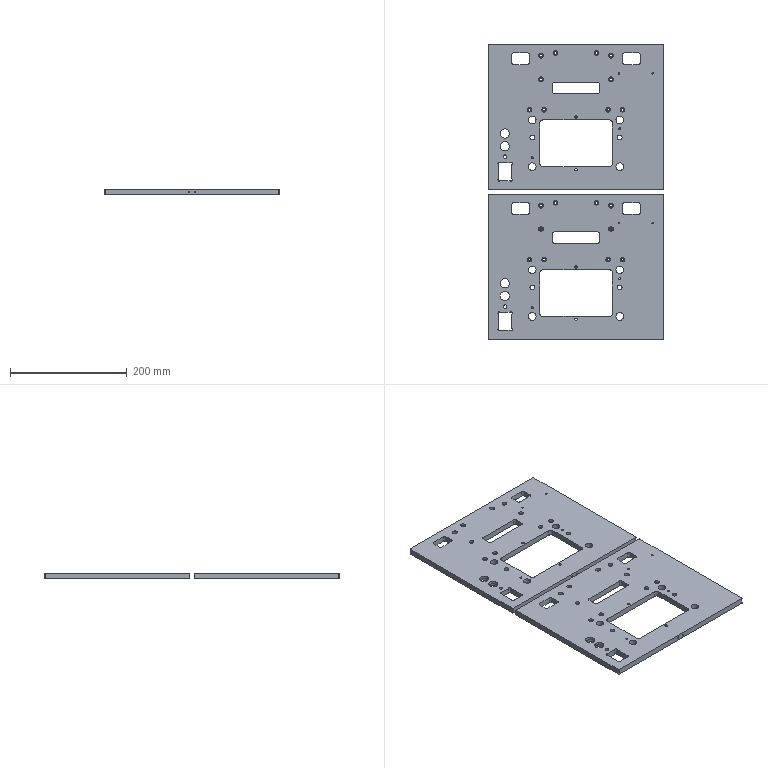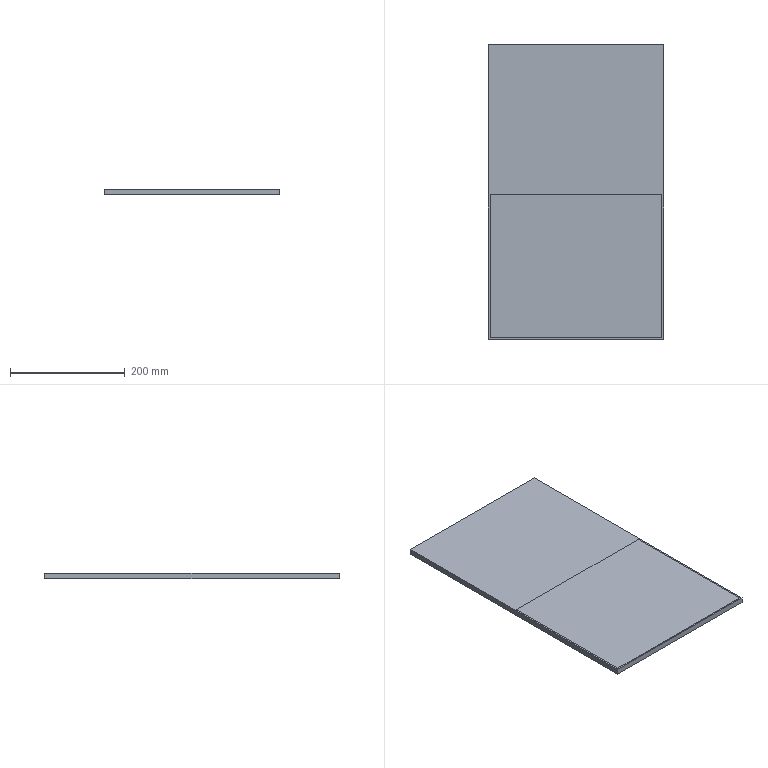CAM job | NX | 3-axis milling, drilling | part box 300 x 507 x 10 mm | stock box 306 x 513 x 10 mm
Tools:
number,name,description,diameter,corner_radius,flute_length,length,flutes
2,D4A45,Milling Tool-5 Parameters,4.0,0.0,2.0,2.0,2
6,D6,Milling Tool-5 Parameters,6.0,0.0,50.0,75.0,2
4,D4,Milling Tool-5 Parameters,4.0,0.0,50.0,75.0,2
13,3.3ZT,Drilling Tool,3.3,0.0,35.0,50.0,2
11,2.5ZT,Drilling Tool,2.5,0.0,35.0,50.0,2
16,4.5ZT,Drilling Tool,4.5,0.0,35.0,50.0,2
14,4.2ZT,Drilling Tool,4.2,0.0,35.0,50.0,2
3,D3,Milling Tool-5 Parameters,3.0,0.0,50.0,75.0,2
Operations:
program,operation,operation_type,tool,method,geometry_group,spindle_rpm,surface_speed,feed_per_tooth,feed_cut,feed_plunge,cut_length_mm,path_length_mm,cut_time_min,machine_time_min
VACUUM1,ZLEVEL_PROFILE_1_COPY_1_COPY_COPY,ZLevelMilling,D4A45,METHOD,A,9500.0,179.0,0.0526,1000.0,100.0,5201.024,17082.464,5.201,6.389
VACUUM1,ZLEVEL_PROFILE_COPY_COPY_1_COPY,ZLevelMilling,D6,METHOD,A,9500.0,179.0,0.1158,2200.0,1000.0,44810.694,45457.393,20.41,20.474
VACUUM1,HOLE_MILLING_COPY,CylinderMilling,D6,METHOD,A,9500.0,179.0,0.0789,1500.0,100.0,1620.814,3835.318,1.081,1.302
VACUUM1,ZLEVEL_PROFILE_COPY_COPY_1_COPY_COPY,ZLevelMilling,D6,METHOD,A,9500.0,179.0,0.0868,1650.0,1000.0,28912.267,30385.631,17.642,17.79
VACUUM1,ZLEVEL_PROFILE_COPY_COPY_COPY_COPY_COPY,ZLevelMilling,D4,MILL_FINISH,A,9500.0,119.0,0.0632,1200.0,1000.0,2228.073,2973.01,1.857,1.932
2,DRILLING_COPY,Operation,D4A45,METHOD,B,5000.0,62.0,0.025,250.0,0.0,140.0,1498.085,0.56,0.6958
2,DRILLING_COPY_COPY_COPY_COPY_COPY,Operation,3.3ZT,METHOD,B,1910.0,21.0,0.0471,180.0,0.0,30.983,283.108,0.1721,0.1973
2,DRILLING_COPY_COPY_COPY_COPY_COPY_COPY_1,Operation,3.3ZT,METHOD,B,1910.0,21.0,0.0471,180.0,0.0,30.983,215.016,0.1721,0.1905
2,DRILLING_COPY_COPY_COPY_COPY_COPY_COPY,Operation,2.5ZT,METHOD,B,1910.0,21.0,0.0471,180.0,0.0,30.502,182.082,0.1695,0.1846
2,DRILLING_COPY_COPY_COPY_COPY_COPY_COPY_COPY_1,Operation,2.5ZT,METHOD,B,1910.0,21.0,0.0471,180.0,0.0,28.506,404.23,0.1584,0.1959
2,DRILLING_COPY_COPY_COPY_COPY_COPY_COPY_COPY,Operation,4.5ZT,METHOD,B,1910.0,21.0,0.0471,180.0,0.0,118.019,680.675,0.6557,0.7119
2,DRILLING_COPY_COPY_COPY_COPY_COPY_COPY_COPY_COPY,Operation,4.2ZT,METHOD,B,1910.0,21.0,0.0471,180.0,0.0,63.047,264.891,0.3503,0.3704
2,ZLEVEL_PROFILE_1_COPY_1_COPY_COPY_COPY,ZLevelMilling,D4A45,METHOD,B,9500.0,179.0,0.0526,1000.0,100.0,2454.682,8526.023,2.455,3.062
2,ZLEVEL_PROFILE_1_COPY_1_COPY_COPY_COPY_COPY,ZLevelMilling,D4A45,METHOD,B,9500.0,179.0,0.0526,1000.0,100.0,547.545,1437.127,0.5475,0.6365
2,ZLEVEL_PROFILE_COPY_COPY_1_COPY_COPY_COPY,ZLevelMilling,D6,METHOD,B,9500.0,179.0,0.0868,1650.0,1000.0,1748.513,1815.513,1.075,1.081
2,HOLE_MILLING_COPY_COPY,CylinderMilling,D6,METHOD,B,9500.0,179.0,0.0789,1500.0,100.0,6647.48,7719.016,4.432,4.539
2,HOLE_MILLING_COPY_COPY_COPY,CylinderMilling,D6,METHOD,B,9500.0,179.0,0.0789,1500.0,100.0,1437.489,1619.489,0.9583,0.9765
2,HOLE_MILLING_COPY_COPY_COPY_COPY,CylinderMilling,D4,METHOD,B,9500.0,179.0,0.0789,1500.0,100.0,95.993,170.494,0.064,0.0714
2,FLOOR_WALL,VolumeBased25DMillingOperation,D4,METHOD,B,9500.0,119.0,0.0526,1000.0,100.0,1508.473,1948.326,1.508,1.552
2,ZLEVEL_PROFILE_COPY_COPY_COPY_COPY_COPY_COPY,ZLevelMilling,D4,MILL_FINISH,B,9500.0,119.0,0.0632,1200.0,1000.0,362.116,1603.284,0.3053,0.4294
2,HOLE_MILLING_1,CylinderMilling,D3,METHOD,B,9500.0,89.0,0.0632,1200.0,100.0,184.718,413.718,0.1539,0.1768
2,CAVITY_MILL_COPY_COPY,CavityMilling,D3,METHOD,B,9500.0,89.0,0.0632,1200.0,1000.0,114.629,768.542,0.1013,0.1667
2,ZLEVEL_PROFILE_1_COPY_1_COPY_COPY_COPY_COPY_COPY,ZLevelMilling,D4A45,METHOD,B,9500.0,179.0,0.0526,1000.0,100.0,73.556,856.148,0.0736,0.1518
2,TOOLOFFSET6,CylinderMilling,D3,METHOD,B,9500.0,179.0,0.0526,1000.0,100.0,44.817,273.817,0.0448,0.0677